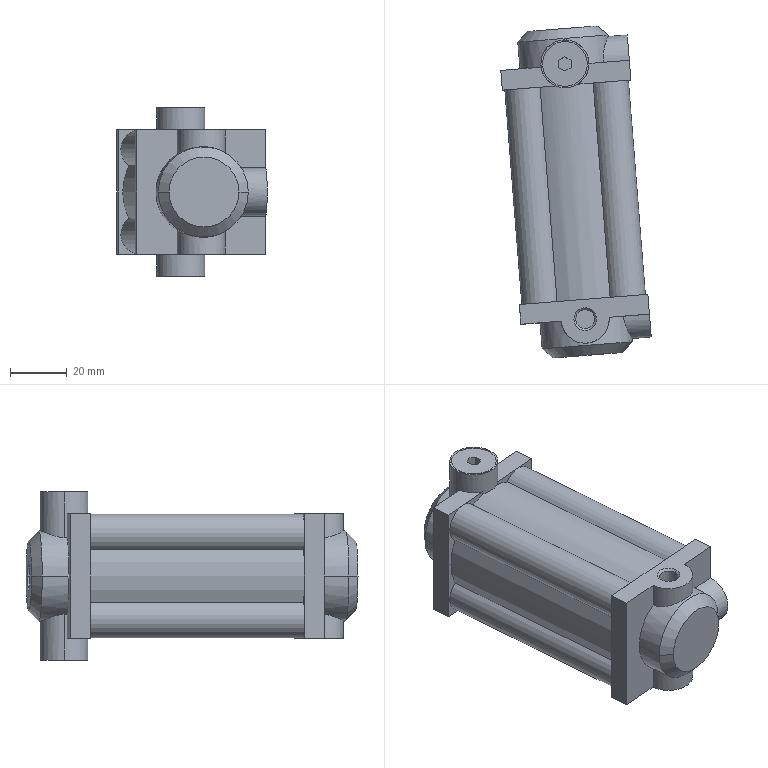Part | STEP file | Sceond_200_APVM0 -5 | 1 solid | 95 faces | box 53.168 x 117.344 x 59.5 mm | volume 144246 mm3 | plane 43 | cylinder 40 | cone 12 | commonest cylinder face diameters 17 x9 13.8 x6 42.5 x5 6.647 x4 8.566 x4 15.8 x4